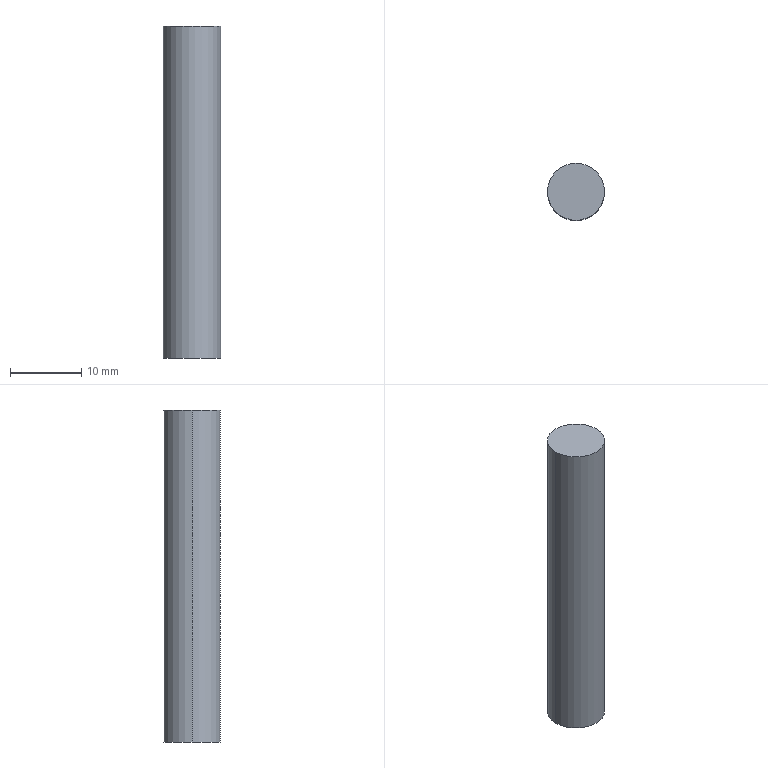Part | SolidWorks | features Extrusion 1 | 1 solid | 4 faces | box 8 x 8 x 46.5 mm | volume 2337 mm3 | cylinder 2 | plane 2 | commonest cylinder face diameters 8 x2
STEP:
#1=CARTESIAN_POINT('',(4.,0.,46.5));
#2=VERTEX_POINT('',#1);
#3=CARTESIAN_POINT('',(-4.,0.,46.5));
#4=VERTEX_POINT('',#3);
#5=CARTESIAN_POINT('',(0.,0.,46.5));
#6=DIRECTION('',(0.,0.,1.));
#7=DIRECTION('',(1.,0.,0.));
#8=AXIS2_PLACEMENT_3D('',#5,#6,#7);
#9=CIRCLE('',#8,4.);
#10=EDGE_CURVE('',#2,#4,#9,.T.);
#11=ORIENTED_EDGE('',*,*,#10,.F.);
#12=CARTESIAN_POINT('',(4.,0.,0.));
#13=VERTEX_POINT('',#12);
#14=CARTESIAN_POINT('',(4.,0.,46.5));
#15=DIRECTION('',(0.,0.,-1.));
#16=VECTOR('',#15,1000.);
#17=LINE('',#14,#16);
#18=EDGE_CURVE('',#2,#13,#17,.T.);
#19=ORIENTED_EDGE('',*,*,#18,.T.);
#20=CARTESIAN_POINT('',(-4.,0.,0.));
#21=VERTEX_POINT('',#20);
#22=CARTESIAN_POINT('',(0.,0.,0.));
#23=DIRECTION('',(0.,0.,1.));
#24=DIRECTION('',(1.,0.,0.));
#25=AXIS2_PLACEMENT_3D('',#22,#23,#24);
#26=CIRCLE('',#25,4.);
#27=EDGE_CURVE('',#13,#21,#26,.T.);
#28=ORIENTED_EDGE('',*,*,#27,.T.);
#29=CARTESIAN_POINT('',(-4.,0.,46.5));
#30=DIRECTION('',(0.,0.,-1.));
#31=VECTOR('',#30,1000.);
#32=LINE('',#29,#31);
#33=EDGE_CURVE('',#4,#21,#32,.T.);
#34=ORIENTED_EDGE('',*,*,#33,.F.);
#35=EDGE_LOOP('',(#11,#19,#28,#34));
#36=FACE_OUTER_BOUND('',#35,.T.);
#37=CARTESIAN_POINT('',(0.,0.,46.5));
#38=DIRECTION('',(0.,0.,-1.));
#39=DIRECTION('',(-1.,0.,0.));
#40=AXIS2_PLACEMENT_3D('',#37,#38,#39);
#41=CYLINDRICAL_SURFACE('',#40,4.);
#42=ADVANCED_FACE('',(#36),#41,.T.);
#43=ORIENTED_EDGE('',*,*,#18,.F.);
#44=CARTESIAN_POINT('',(0.,0.,46.5));
#45=DIRECTION('',(0.,0.,1.));
#46=DIRECTION('',(1.,0.,0.));
#47=AXIS2_PLACEMENT_3D('',#44,#45,#46);
#48=CIRCLE('',#47,4.);
#49=EDGE_CURVE('',#4,#2,#48,.T.);
#50=ORIENTED_EDGE('',*,*,#49,.F.);
#51=ORIENTED_EDGE('',*,*,#33,.T.);
#52=CARTESIAN_POINT('',(0.,0.,0.));
#53=DIRECTION('',(0.,0.,1.));
#54=DIRECTION('',(1.,0.,0.));
#55=AXIS2_PLACEMENT_3D('',#52,#53,#54);
#56=CIRCLE('',#55,4.);
#57=EDGE_CURVE('',#21,#13,#56,.T.);
#58=ORIENTED_EDGE('',*,*,#57,.T.);
#59=EDGE_LOOP('',(#43,#50,#51,#58));
#60=FACE_OUTER_BOUND('',#59,.T.);
#61=CARTESIAN_POINT('',(0.,0.,46.5));
#62=DIRECTION('',(0.,0.,-1.));
#63=DIRECTION('',(-1.,0.,0.));
#64=AXIS2_PLACEMENT_3D('',#61,#62,#63);
#65=CYLINDRICAL_SURFACE('',#64,4.);
#66=ADVANCED_FACE('',(#60),#65,.T.);
#67=ORIENTED_EDGE('',*,*,#49,.T.);
#68=ORIENTED_EDGE('',*,*,#10,.T.);
#69=EDGE_LOOP('',(#67,#68));
#70=FACE_OUTER_BOUND('',#69,.T.);
#71=CARTESIAN_POINT('',(0.,0.,46.5));
#72=DIRECTION('',(0.,0.,1.));
#73=DIRECTION('',(1.,0.,0.));
#74=AXIS2_PLACEMENT_3D('',#71,#72,#73);
#75=PLANE('',#74);
#76=ADVANCED_FACE('',(#70),#75,.T.);
#77=ORIENTED_EDGE('',*,*,#57,.F.);
#78=ORIENTED_EDGE('',*,*,#27,.F.);
#79=EDGE_LOOP('',(#77,#78));
#80=FACE_OUTER_BOUND('',#79,.T.);
#81=CARTESIAN_POINT('',(0.,0.,0.));
#82=DIRECTION('',(0.,0.,1.));
#83=DIRECTION('',(1.,0.,0.));
#84=AXIS2_PLACEMENT_3D('',#81,#82,#83);
#85=PLANE('',#84);
#86=ADVANCED_FACE('',(#80),#85,.F.);
#87=CLOSED_SHELL('',(#42,#66,#76,#86));
#88=MANIFOLD_SOLID_BREP('',#87);
#89=CARTESIAN_POINT('',(0.,0.,0.));
#90=DIRECTION('',(0.,0.,1.));
#91=DIRECTION('',(1.,0.,0.));
#92=AXIS2_PLACEMENT_3D('',#89,#90,#91);
#93=(LENGTH_UNIT()NAMED_UNIT(*)SI_UNIT(.MILLI.,.METRE.));
#94=UNCERTAINTY_MEASURE_WITH_UNIT(LENGTH_MEASURE(0.00001),#93,'','');
#95=(NAMED_UNIT(*)PLANE_ANGLE_UNIT()SI_UNIT($,.RADIAN.));
#96=(NAMED_UNIT(*)SI_UNIT($,.STERADIAN.)SOLID_ANGLE_UNIT());
#97=(GEOMETRIC_REPRESENTATION_CONTEXT(3)GLOBAL_UNCERTAINTY_ASSIGNED_CONTEXT((#94))GLOBAL_UNIT_ASSIGNED_CONTEXT((#93,#95,#96))REPRESENTATION_CONTEXT('',''));
#98=ADVANCED_BREP_SHAPE_REPRESENTATION('',(#88,#92),#97);